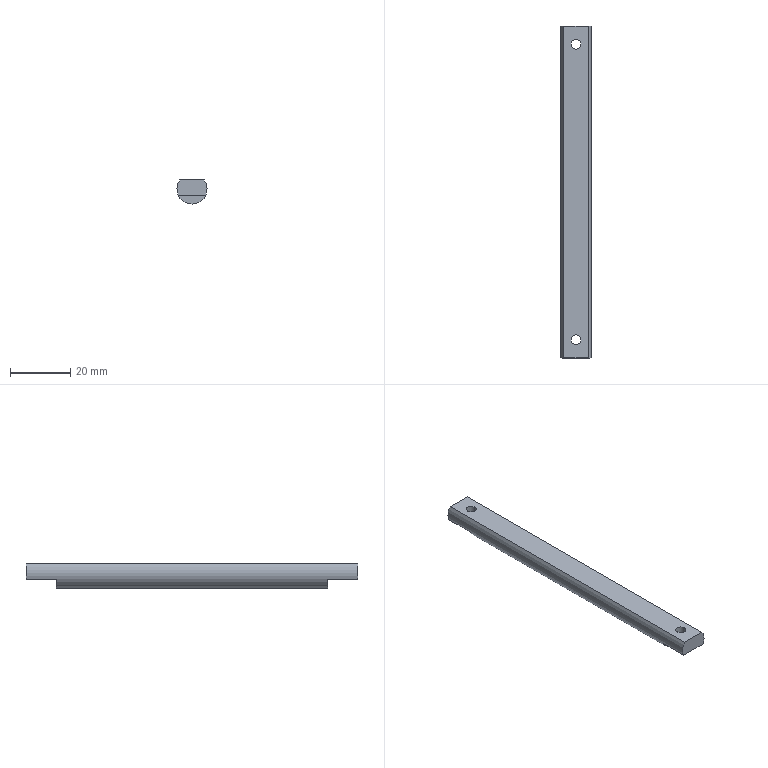Part | SolidWorks | features ICE 2, Extrusion 1, HoleWzd 1, MirrorPattern 1 | 1 solid | 13 faces | box 10 x 110 x 8 mm | volume 6927 mm3 | plane 7 | cylinder 6 | commonest cylinder face diameters 3.3 x4 10 x2
STEP:
#1=CARTESIAN_POINT('',(1.65,104.,3.));
#2=VERTEX_POINT('',#1);
#3=CARTESIAN_POINT('',(-1.65,104.,3.));
#4=VERTEX_POINT('',#3);
#5=CARTESIAN_POINT('',(0.,104.,3.));
#6=DIRECTION('',(0.,0.,-1.));
#7=DIRECTION('',(-1.,0.,0.));
#8=AXIS2_PLACEMENT_3D('',#5,#6,#7);
#9=CIRCLE('',#8,1.65);
#10=EDGE_CURVE('',#2,#4,#9,.T.);
#11=ORIENTED_EDGE('',*,*,#10,.F.);
#12=CARTESIAN_POINT('',(1.65,104.,-2.));
#13=VERTEX_POINT('',#12);
#14=CARTESIAN_POINT('',(1.65,104.,-2.));
#15=DIRECTION('',(0.,0.,-1.));
#16=VECTOR('',#15,1000.);
#17=LINE('',#14,#16);
#18=EDGE_CURVE('',#2,#13,#17,.T.);
#19=ORIENTED_EDGE('',*,*,#18,.T.);
#20=CARTESIAN_POINT('',(-1.65,104.,-2.));
#21=VERTEX_POINT('',#20);
#22=CARTESIAN_POINT('',(0.,104.,-2.));
#23=DIRECTION('',(0.,0.,-1.));
#24=DIRECTION('',(-1.,0.,0.));
#25=AXIS2_PLACEMENT_3D('',#22,#23,#24);
#26=CIRCLE('',#25,1.65);
#27=EDGE_CURVE('',#13,#21,#26,.T.);
#28=ORIENTED_EDGE('',*,*,#27,.T.);
#29=CARTESIAN_POINT('',(-1.65,104.,-2.));
#30=DIRECTION('',(0.,0.,-1.));
#31=VECTOR('',#30,1000.);
#32=LINE('',#29,#31);
#33=EDGE_CURVE('',#4,#21,#32,.T.);
#34=ORIENTED_EDGE('',*,*,#33,.F.);
#35=EDGE_LOOP('',(#11,#19,#28,#34));
#36=FACE_OUTER_BOUND('',#35,.T.);
#37=CARTESIAN_POINT('',(0.,104.,-2.));
#38=DIRECTION('',(0.,0.,-1.));
#39=DIRECTION('',(-1.,0.,0.));
#40=AXIS2_PLACEMENT_3D('',#37,#38,#39);
#41=CYLINDRICAL_SURFACE('',#40,1.65);
#42=ADVANCED_FACE('',(#36),#41,.F.);
#43=CARTESIAN_POINT('',(1.65,6.,3.));
#44=VERTEX_POINT('',#43);
#45=CARTESIAN_POINT('',(-1.65,6.,3.));
#46=VERTEX_POINT('',#45);
#47=CARTESIAN_POINT('',(0.,6.,3.));
#48=DIRECTION('',(0.,0.,-1.));
#49=DIRECTION('',(-1.,0.,0.));
#50=AXIS2_PLACEMENT_3D('',#47,#48,#49);
#51=CIRCLE('',#50,1.65);
#52=EDGE_CURVE('',#44,#46,#51,.T.);
#53=ORIENTED_EDGE('',*,*,#52,.F.);
#54=CARTESIAN_POINT('',(1.65,6.,-2.));
#55=VERTEX_POINT('',#54);
#56=CARTESIAN_POINT('',(1.65,6.,-2.));
#57=DIRECTION('',(0.,0.,-1.));
#58=VECTOR('',#57,1000.);
#59=LINE('',#56,#58);
#60=EDGE_CURVE('',#44,#55,#59,.T.);
#61=ORIENTED_EDGE('',*,*,#60,.T.);
#62=CARTESIAN_POINT('',(-1.65,6.,-2.));
#63=VERTEX_POINT('',#62);
#64=CARTESIAN_POINT('',(0.,6.,-2.));
#65=DIRECTION('',(0.,0.,-1.));
#66=DIRECTION('',(-1.,0.,0.));
#67=AXIS2_PLACEMENT_3D('',#64,#65,#66);
#68=CIRCLE('',#67,1.65);
#69=EDGE_CURVE('',#55,#63,#68,.T.);
#70=ORIENTED_EDGE('',*,*,#69,.T.);
#71=CARTESIAN_POINT('',(-1.65,6.,-2.));
#72=DIRECTION('',(0.,0.,-1.));
#73=VECTOR('',#72,1000.);
#74=LINE('',#71,#73);
#75=EDGE_CURVE('',#46,#63,#74,.T.);
#76=ORIENTED_EDGE('',*,*,#75,.F.);
#77=EDGE_LOOP('',(#53,#61,#70,#76));
#78=FACE_OUTER_BOUND('',#77,.T.);
#79=CARTESIAN_POINT('',(0.,6.,-2.));
#80=DIRECTION('',(0.,0.,-1.));
#81=DIRECTION('',(-1.,0.,0.));
#82=AXIS2_PLACEMENT_3D('',#79,#80,#81);
#83=CYLINDRICAL_SURFACE('',#82,1.65);
#84=ADVANCED_FACE('',(#78),#83,.F.);
#85=CARTESIAN_POINT('',(0.,100.,-5.));
#86=VERTEX_POINT('',#85);
#87=CARTESIAN_POINT('',(-4.583,100.,-2.));
#88=VERTEX_POINT('',#87);
#89=CARTESIAN_POINT('',(0.,100.,0.));
#90=DIRECTION('',(0.,1.,0.));
#91=DIRECTION('',(0.,0.,1.));
#92=AXIS2_PLACEMENT_3D('',#89,#90,#91);
#93=CIRCLE('',#92,5.);
#94=EDGE_CURVE('',#86,#88,#93,.T.);
#95=ORIENTED_EDGE('',*,*,#94,.F.);
#96=CARTESIAN_POINT('',(0.,10.,-5.));
#97=VERTEX_POINT('',#96);
#98=CARTESIAN_POINT('',(0.,110.,-5.));
#99=DIRECTION('',(0.,-1.,0.));
#100=VECTOR('',#99,1000.);
#101=LINE('',#98,#100);
#102=EDGE_CURVE('',#86,#97,#101,.T.);
#103=ORIENTED_EDGE('',*,*,#102,.T.);
#104=CARTESIAN_POINT('',(-4.583,10.,-2.));
#105=VERTEX_POINT('',#104);
#106=CARTESIAN_POINT('',(0.,10.,0.));
#107=DIRECTION('',(0.,1.,0.));
#108=DIRECTION('',(0.,0.,1.));
#109=AXIS2_PLACEMENT_3D('',#106,#107,#108);
#110=CIRCLE('',#109,5.);
#111=EDGE_CURVE('',#97,#105,#110,.T.);
#112=ORIENTED_EDGE('',*,*,#111,.T.);
#113=CARTESIAN_POINT('',(-4.583,0.,-2.));
#114=VERTEX_POINT('',#113);
#115=CARTESIAN_POINT('',(-4.583,10.,-2.));
#116=DIRECTION('',(0.,-1.,0.));
#117=VECTOR('',#116,1000.);
#118=LINE('',#115,#117);
#119=EDGE_CURVE('',#105,#114,#118,.T.);
#120=ORIENTED_EDGE('',*,*,#119,.T.);
#121=CARTESIAN_POINT('',(-4.,0.,3.));
#122=VERTEX_POINT('',#121);
#123=CARTESIAN_POINT('',(0.,0.,0.));
#124=DIRECTION('',(0.,1.,0.));
#125=DIRECTION('',(0.,0.,1.));
#126=AXIS2_PLACEMENT_3D('',#123,#124,#125);
#127=CIRCLE('',#126,5.);
#128=EDGE_CURVE('',#114,#122,#127,.T.);
#129=ORIENTED_EDGE('',*,*,#128,.T.);
#130=CARTESIAN_POINT('',(-4.,110.,3.));
#131=VERTEX_POINT('',#130);
#132=CARTESIAN_POINT('',(-4.,0.,3.));
#133=DIRECTION('',(0.,1.,0.));
#134=VECTOR('',#133,1000.);
#135=LINE('',#132,#134);
#136=EDGE_CURVE('',#122,#131,#135,.T.);
#137=ORIENTED_EDGE('',*,*,#136,.T.);
#138=CARTESIAN_POINT('',(-4.583,110.,-2.));
#139=VERTEX_POINT('',#138);
#140=CARTESIAN_POINT('',(0.,110.,0.));
#141=DIRECTION('',(0.,1.,0.));
#142=DIRECTION('',(0.,0.,1.));
#143=AXIS2_PLACEMENT_3D('',#140,#141,#142);
#144=CIRCLE('',#143,5.);
#145=EDGE_CURVE('',#139,#131,#144,.T.);
#146=ORIENTED_EDGE('',*,*,#145,.F.);
#147=CARTESIAN_POINT('',(-4.583,100.,-2.));
#148=DIRECTION('',(0.,1.,0.));
#149=VECTOR('',#148,1000.);
#150=LINE('',#147,#149);
#151=EDGE_CURVE('',#88,#139,#150,.T.);
#152=ORIENTED_EDGE('',*,*,#151,.F.);
#153=EDGE_LOOP('',(#95,#103,#112,#120,#129,#137,#146,#152));
#154=FACE_OUTER_BOUND('',#153,.T.);
#155=CARTESIAN_POINT('',(0.,110.,0.));
#156=DIRECTION('',(0.,-1.,0.));
#157=DIRECTION('',(0.,0.,-1.));
#158=AXIS2_PLACEMENT_3D('',#155,#156,#157);
#159=CYLINDRICAL_SURFACE('',#158,5.);
#160=ADVANCED_FACE('',(#154),#159,.T.);
#161=ORIENTED_EDGE('',*,*,#102,.F.);
#162=CARTESIAN_POINT('',(4.583,100.,-2.));
#163=VERTEX_POINT('',#162);
#164=CARTESIAN_POINT('',(0.,100.,0.));
#165=DIRECTION('',(0.,1.,0.));
#166=DIRECTION('',(0.,0.,1.));
#167=AXIS2_PLACEMENT_3D('',#164,#165,#166);
#168=CIRCLE('',#167,5.);
#169=EDGE_CURVE('',#163,#86,#168,.T.);
#170=ORIENTED_EDGE('',*,*,#169,.F.);
#171=CARTESIAN_POINT('',(4.583,110.,-2.));
#172=VERTEX_POINT('',#171);
#173=CARTESIAN_POINT('',(4.583,100.,-2.));
#174=DIRECTION('',(0.,1.,0.));
#175=VECTOR('',#174,1000.);
#176=LINE('',#173,#175);
#177=EDGE_CURVE('',#163,#172,#176,.T.);
#178=ORIENTED_EDGE('',*,*,#177,.T.);
#179=CARTESIAN_POINT('',(4.,110.,3.));
#180=VERTEX_POINT('',#179);
#181=CARTESIAN_POINT('',(0.,110.,0.));
#182=DIRECTION('',(0.,1.,0.));
#183=DIRECTION('',(0.,0.,1.));
#184=AXIS2_PLACEMENT_3D('',#181,#182,#183);
#185=CIRCLE('',#184,5.);
#186=EDGE_CURVE('',#180,#172,#185,.T.);
#187=ORIENTED_EDGE('',*,*,#186,.F.);
#188=CARTESIAN_POINT('',(4.,0.,3.));
#189=VERTEX_POINT('',#188);
#190=CARTESIAN_POINT('',(4.,0.,3.));
#191=DIRECTION('',(0.,1.,0.));
#192=VECTOR('',#191,1000.);
#193=LINE('',#190,#192);
#194=EDGE_CURVE('',#189,#180,#193,.T.);
#195=ORIENTED_EDGE('',*,*,#194,.F.);
#196=CARTESIAN_POINT('',(4.583,0.,-2.));
#197=VERTEX_POINT('',#196);
#198=CARTESIAN_POINT('',(0.,0.,0.));
#199=DIRECTION('',(0.,1.,0.));
#200=DIRECTION('',(0.,0.,1.));
#201=AXIS2_PLACEMENT_3D('',#198,#199,#200);
#202=CIRCLE('',#201,5.);
#203=EDGE_CURVE('',#189,#197,#202,.T.);
#204=ORIENTED_EDGE('',*,*,#203,.T.);
#205=CARTESIAN_POINT('',(4.583,10.,-2.));
#206=VERTEX_POINT('',#205);
#207=CARTESIAN_POINT('',(4.583,10.,-2.));
#208=DIRECTION('',(0.,-1.,0.));
#209=VECTOR('',#208,1000.);
#210=LINE('',#207,#209);
#211=EDGE_CURVE('',#206,#197,#210,.T.);
#212=ORIENTED_EDGE('',*,*,#211,.F.);
#213=CARTESIAN_POINT('',(0.,10.,0.));
#214=DIRECTION('',(0.,1.,0.));
#215=DIRECTION('',(0.,0.,1.));
#216=AXIS2_PLACEMENT_3D('',#213,#214,#215);
#217=CIRCLE('',#216,5.);
#218=EDGE_CURVE('',#206,#97,#217,.T.);
#219=ORIENTED_EDGE('',*,*,#218,.T.);
#220=EDGE_LOOP('',(#161,#170,#178,#187,#195,#204,#212,#219));
#221=FACE_OUTER_BOUND('',#220,.T.);
#222=CARTESIAN_POINT('',(0.,110.,0.));
#223=DIRECTION('',(0.,-1.,0.));
#224=DIRECTION('',(0.,0.,-1.));
#225=AXIS2_PLACEMENT_3D('',#222,#223,#224);
#226=CYLINDRICAL_SURFACE('',#225,5.);
#227=ADVANCED_FACE('',(#221),#226,.T.);
#228=CARTESIAN_POINT('',(-4.583,0.,-2.));
#229=DIRECTION('',(1.,0.,0.));
#230=VECTOR('',#229,1000.);
#231=LINE('',#228,#230);
#232=EDGE_CURVE('',#114,#197,#231,.T.);
#233=ORIENTED_EDGE('',*,*,#232,.T.);
#234=ORIENTED_EDGE('',*,*,#203,.F.);
#235=CARTESIAN_POINT('',(-4.,0.,3.));
#236=DIRECTION('',(-1.,0.,0.));
#237=VECTOR('',#236,1000.);
#238=LINE('',#235,#237);
#239=EDGE_CURVE('',#189,#122,#238,.T.);
#240=ORIENTED_EDGE('',*,*,#239,.T.);
#241=ORIENTED_EDGE('',*,*,#128,.F.);
#242=EDGE_LOOP('',(#233,#234,#240,#241));
#243=FACE_OUTER_BOUND('',#242,.T.);
#244=CARTESIAN_POINT('',(0.,0.,0.));
#245=DIRECTION('',(0.,1.,0.));
#246=DIRECTION('',(0.,0.,1.));
#247=AXIS2_PLACEMENT_3D('',#244,#245,#246);
#248=PLANE('',#247);
#249=ADVANCED_FACE('',(#243),#248,.F.);
#250=CARTESIAN_POINT('',(-4.583,110.,-2.));
#251=DIRECTION('',(1.,0.,0.));
#252=VECTOR('',#251,1000.);
#253=LINE('',#250,#252);
#254=EDGE_CURVE('',#139,#172,#253,.T.);
#255=ORIENTED_EDGE('',*,*,#254,.F.);
#256=ORIENTED_EDGE('',*,*,#145,.T.);
#257=CARTESIAN_POINT('',(-4.,110.,3.));
#258=DIRECTION('',(-1.,0.,0.));
#259=VECTOR('',#258,1000.);
#260=LINE('',#257,#259);
#261=EDGE_CURVE('',#180,#131,#260,.T.);
#262=ORIENTED_EDGE('',*,*,#261,.F.);
#263=ORIENTED_EDGE('',*,*,#186,.T.);
#264=EDGE_LOOP('',(#255,#256,#262,#263));
#265=FACE_OUTER_BOUND('',#264,.T.);
#266=CARTESIAN_POINT('',(0.,110.,0.));
#267=DIRECTION('',(0.,1.,0.));
#268=DIRECTION('',(0.,0.,1.));
#269=AXIS2_PLACEMENT_3D('',#266,#267,#268);
#270=PLANE('',#269);
#271=ADVANCED_FACE('',(#265),#270,.T.);
#272=CARTESIAN_POINT('',(0.,104.,3.));
#273=DIRECTION('',(0.,0.,-1.));
#274=DIRECTION('',(-1.,0.,0.));
#275=AXIS2_PLACEMENT_3D('',#272,#273,#274);
#276=CIRCLE('',#275,1.65);
#277=EDGE_CURVE('',#4,#2,#276,.T.);
#278=ORIENTED_EDGE('',*,*,#277,.T.);
#279=ORIENTED_EDGE('',*,*,#10,.T.);
#280=EDGE_LOOP('',(#278,#279));
#281=FACE_BOUND('',#280,.T.);
#282=CARTESIAN_POINT('',(0.,6.,3.));
#283=DIRECTION('',(0.,0.,-1.));
#284=DIRECTION('',(-1.,0.,0.));
#285=AXIS2_PLACEMENT_3D('',#282,#283,#284);
#286=CIRCLE('',#285,1.65);
#287=EDGE_CURVE('',#46,#44,#286,.T.);
#288=ORIENTED_EDGE('',*,*,#287,.T.);
#289=ORIENTED_EDGE('',*,*,#52,.T.);
#290=EDGE_LOOP('',(#288,#289));
#291=FACE_BOUND('',#290,.T.);
#292=ORIENTED_EDGE('',*,*,#261,.T.);
#293=ORIENTED_EDGE('',*,*,#136,.F.);
#294=ORIENTED_EDGE('',*,*,#239,.F.);
#295=ORIENTED_EDGE('',*,*,#194,.T.);
#296=EDGE_LOOP('',(#292,#293,#294,#295));
#297=FACE_OUTER_BOUND('',#296,.T.);
#298=CARTESIAN_POINT('',(-4.,0.,3.));
#299=DIRECTION('',(0.,0.,-1.));
#300=DIRECTION('',(-1.,0.,0.));
#301=AXIS2_PLACEMENT_3D('',#298,#299,#300);
#302=PLANE('',#301);
#303=ADVANCED_FACE('',(#281,#291,#297),#302,.F.);
#304=CARTESIAN_POINT('',(0.,104.,-2.));
#305=DIRECTION('',(0.,0.,-1.));
#306=DIRECTION('',(-1.,0.,0.));
#307=AXIS2_PLACEMENT_3D('',#304,#305,#306);
#308=CIRCLE('',#307,1.65);
#309=EDGE_CURVE('',#21,#13,#308,.T.);
#310=ORIENTED_EDGE('',*,*,#309,.F.);
#311=ORIENTED_EDGE('',*,*,#27,.F.);
#312=EDGE_LOOP('',(#310,#311));
#313=FACE_BOUND('',#312,.T.);
#314=ORIENTED_EDGE('',*,*,#254,.T.);
#315=ORIENTED_EDGE('',*,*,#177,.F.);
#316=CARTESIAN_POINT('',(-4.583,100.,-2.));
#317=DIRECTION('',(1.,0.,0.));
#318=VECTOR('',#317,1000.);
#319=LINE('',#316,#318);
#320=EDGE_CURVE('',#88,#163,#319,.T.);
#321=ORIENTED_EDGE('',*,*,#320,.F.);
#322=ORIENTED_EDGE('',*,*,#151,.T.);
#323=EDGE_LOOP('',(#314,#315,#321,#322));
#324=FACE_OUTER_BOUND('',#323,.T.);
#325=CARTESIAN_POINT('',(-4.583,100.,-2.));
#326=DIRECTION('',(0.,0.,1.));
#327=DIRECTION('',(1.,0.,0.));
#328=AXIS2_PLACEMENT_3D('',#325,#326,#327);
#329=PLANE('',#328);
#330=ADVANCED_FACE('',(#313,#324),#329,.F.);
#331=ORIENTED_EDGE('',*,*,#169,.T.);
#332=ORIENTED_EDGE('',*,*,#94,.T.);
#333=ORIENTED_EDGE('',*,*,#320,.T.);
#334=EDGE_LOOP('',(#331,#332,#333));
#335=FACE_OUTER_BOUND('',#334,.T.);
#336=CARTESIAN_POINT('',(0.,100.,0.));
#337=DIRECTION('',(0.,1.,0.));
#338=DIRECTION('',(0.,0.,1.));
#339=AXIS2_PLACEMENT_3D('',#336,#337,#338);
#340=PLANE('',#339);
#341=ADVANCED_FACE('',(#335),#340,.T.);
#342=CARTESIAN_POINT('',(0.,6.,-2.));
#343=DIRECTION('',(0.,0.,-1.));
#344=DIRECTION('',(-1.,0.,0.));
#345=AXIS2_PLACEMENT_3D('',#342,#343,#344);
#346=CIRCLE('',#345,1.65);
#347=EDGE_CURVE('',#63,#55,#346,.T.);
#348=ORIENTED_EDGE('',*,*,#347,.F.);
#349=ORIENTED_EDGE('',*,*,#69,.F.);
#350=EDGE_LOOP('',(#348,#349));
#351=FACE_BOUND('',#350,.T.);
#352=ORIENTED_EDGE('',*,*,#232,.F.);
#353=ORIENTED_EDGE('',*,*,#119,.F.);
#354=CARTESIAN_POINT('',(-4.583,10.,-2.));
#355=DIRECTION('',(1.,0.,0.));
#356=VECTOR('',#355,1000.);
#357=LINE('',#354,#356);
#358=EDGE_CURVE('',#105,#206,#357,.T.);
#359=ORIENTED_EDGE('',*,*,#358,.T.);
#360=ORIENTED_EDGE('',*,*,#211,.T.);
#361=EDGE_LOOP('',(#352,#353,#359,#360));
#362=FACE_OUTER_BOUND('',#361,.T.);
#363=CARTESIAN_POINT('',(-4.583,10.,-2.));
#364=DIRECTION('',(0.,0.,-1.));
#365=DIRECTION('',(-1.,0.,0.));
#366=AXIS2_PLACEMENT_3D('',#363,#364,#365);
#367=PLANE('',#366);
#368=ADVANCED_FACE('',(#351,#362),#367,.T.);
#369=ORIENTED_EDGE('',*,*,#218,.F.);
#370=ORIENTED_EDGE('',*,*,#358,.F.);
#371=ORIENTED_EDGE('',*,*,#111,.F.);
#372=EDGE_LOOP('',(#369,#370,#371));
#373=FACE_OUTER_BOUND('',#372,.T.);
#374=CARTESIAN_POINT('',(0.,10.,0.));
#375=DIRECTION('',(0.,-1.,0.));
#376=DIRECTION('',(0.,0.,1.));
#377=AXIS2_PLACEMENT_3D('',#374,#375,#376);
#378=PLANE('',#377);
#379=ADVANCED_FACE('',(#373),#378,.T.);
#380=ORIENTED_EDGE('',*,*,#60,.F.);
#381=ORIENTED_EDGE('',*,*,#287,.F.);
#382=ORIENTED_EDGE('',*,*,#75,.T.);
#383=ORIENTED_EDGE('',*,*,#347,.T.);
#384=EDGE_LOOP('',(#380,#381,#382,#383));
#385=FACE_OUTER_BOUND('',#384,.T.);
#386=CARTESIAN_POINT('',(0.,6.,-2.));
#387=DIRECTION('',(0.,0.,-1.));
#388=DIRECTION('',(-1.,0.,0.));
#389=AXIS2_PLACEMENT_3D('',#386,#387,#388);
#390=CYLINDRICAL_SURFACE('',#389,1.65);
#391=ADVANCED_FACE('',(#385),#390,.F.);
#392=ORIENTED_EDGE('',*,*,#18,.F.);
#393=ORIENTED_EDGE('',*,*,#277,.F.);
#394=ORIENTED_EDGE('',*,*,#33,.T.);
#395=ORIENTED_EDGE('',*,*,#309,.T.);
#396=EDGE_LOOP('',(#392,#393,#394,#395));
#397=FACE_OUTER_BOUND('',#396,.T.);
#398=CARTESIAN_POINT('',(0.,104.,-2.));
#399=DIRECTION('',(0.,0.,-1.));
#400=DIRECTION('',(-1.,0.,0.));
#401=AXIS2_PLACEMENT_3D('',#398,#399,#400);
#402=CYLINDRICAL_SURFACE('',#401,1.65);
#403=ADVANCED_FACE('',(#397),#402,.F.);
#404=CLOSED_SHELL('',(#42,#84,#160,#227,#249,#271,#303,#330,#341,#368,#379,#391,#403));
#405=MANIFOLD_SOLID_BREP('',#404);
#406=CARTESIAN_POINT('',(0.,0.,0.));
#407=DIRECTION('',(0.,0.,1.));
#408=DIRECTION('',(1.,0.,0.));
#409=AXIS2_PLACEMENT_3D('',#406,#407,#408);
#410=(LENGTH_UNIT()NAMED_UNIT(*)SI_UNIT(.MILLI.,.METRE.));
#411=UNCERTAINTY_MEASURE_WITH_UNIT(LENGTH_MEASURE(0.00001),#410,'','');
#412=(NAMED_UNIT(*)PLANE_ANGLE_UNIT()SI_UNIT($,.RADIAN.));
#413=(NAMED_UNIT(*)SI_UNIT($,.STERADIAN.)SOLID_ANGLE_UNIT());
#414=(GEOMETRIC_REPRESENTATION_CONTEXT(3)GLOBAL_UNCERTAINTY_ASSIGNED_CONTEXT((#411))GLOBAL_UNIT_ASSIGNED_CONTEXT((#410,#412,#413))REPRESENTATION_CONTEXT('',''));
#415=ADVANCED_BREP_SHAPE_REPRESENTATION('',(#405,#409),#414);